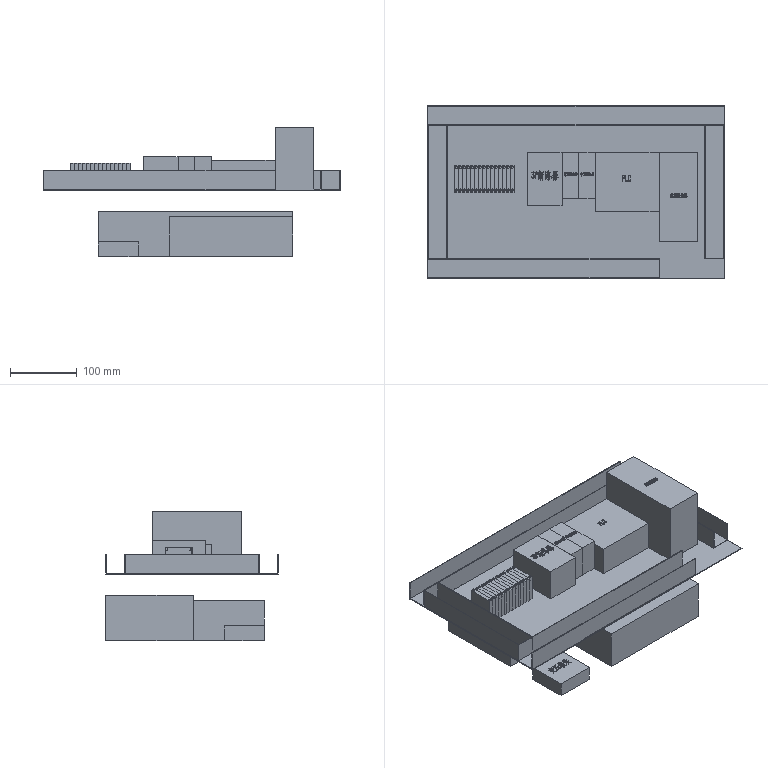Part | SolidWorks | features BaseBody 28 | 28 solids | 4085 faces | volume 5761098 mm3 | plane 2958 | spline 1067 | cylinder 60 | commonest cylinder face diameters 3 x60